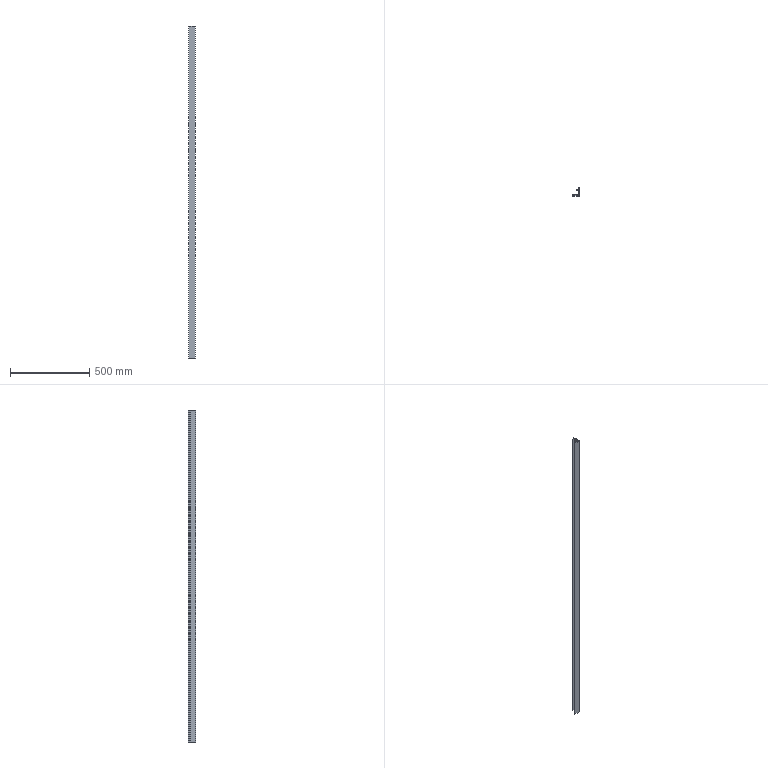Part | SolidWorks | features Extrusion 1, ICE 1 | 2 solids | 14 faces | box 43 x 50 x 2090 mm | volume 1054401 mm3 | plane 14
STEP:
#1=CARTESIAN_POINT('',(-43.,5.,-1045.));
#2=VERTEX_POINT('',#1);
#3=CARTESIAN_POINT('',(-43.,0.,-1045.));
#4=VERTEX_POINT('',#3);
#5=CARTESIAN_POINT('',(-43.,5.,-1045.));
#6=DIRECTION('',(0.,-1.,0.));
#7=VECTOR('',#6,1000.);
#8=LINE('',#5,#7);
#9=EDGE_CURVE('',#2,#4,#8,.T.);
#10=ORIENTED_EDGE('',*,*,#9,.T.);
#11=CARTESIAN_POINT('',(-43.,0.,1045.));
#12=VERTEX_POINT('',#11);
#13=CARTESIAN_POINT('',(-43.,0.,1045.));
#14=DIRECTION('',(0.,0.,-1.));
#15=VECTOR('',#14,1000.);
#16=LINE('',#13,#15);
#17=EDGE_CURVE('',#12,#4,#16,.T.);
#18=ORIENTED_EDGE('',*,*,#17,.F.);
#19=CARTESIAN_POINT('',(-43.,5.,1045.));
#20=VERTEX_POINT('',#19);
#21=CARTESIAN_POINT('',(-43.,5.,1045.));
#22=DIRECTION('',(0.,-1.,0.));
#23=VECTOR('',#22,1000.);
#24=LINE('',#21,#23);
#25=EDGE_CURVE('',#20,#12,#24,.T.);
#26=ORIENTED_EDGE('',*,*,#25,.F.);
#27=CARTESIAN_POINT('',(-43.,5.,1045.));
#28=DIRECTION('',(0.,0.,-1.));
#29=VECTOR('',#28,1000.);
#30=LINE('',#27,#29);
#31=EDGE_CURVE('',#20,#2,#30,.T.);
#32=ORIENTED_EDGE('',*,*,#31,.T.);
#33=EDGE_LOOP('',(#10,#18,#26,#32));
#34=FACE_OUTER_BOUND('',#33,.T.);
#35=CARTESIAN_POINT('',(-43.,5.,1045.));
#36=DIRECTION('',(1.,0.,0.));
#37=DIRECTION('',(0.,0.,-1.));
#38=AXIS2_PLACEMENT_3D('',#35,#36,#37);
#39=PLANE('',#38);
#40=ADVANCED_FACE('',(#34),#39,.F.);
#41=CARTESIAN_POINT('',(0.,0.,-1045.));
#42=VERTEX_POINT('',#41);
#43=CARTESIAN_POINT('',(-43.,0.,-1045.));
#44=DIRECTION('',(1.,0.,0.));
#45=VECTOR('',#44,1000.);
#46=LINE('',#43,#45);
#47=EDGE_CURVE('',#4,#42,#46,.T.);
#48=ORIENTED_EDGE('',*,*,#47,.T.);
#49=CARTESIAN_POINT('',(0.,0.,1045.));
#50=VERTEX_POINT('',#49);
#51=CARTESIAN_POINT('',(0.,0.,1045.));
#52=DIRECTION('',(0.,0.,-1.));
#53=VECTOR('',#52,1000.);
#54=LINE('',#51,#53);
#55=EDGE_CURVE('',#50,#42,#54,.T.);
#56=ORIENTED_EDGE('',*,*,#55,.F.);
#57=CARTESIAN_POINT('',(-43.,0.,1045.));
#58=DIRECTION('',(1.,0.,0.));
#59=VECTOR('',#58,1000.);
#60=LINE('',#57,#59);
#61=EDGE_CURVE('',#12,#50,#60,.T.);
#62=ORIENTED_EDGE('',*,*,#61,.F.);
#63=ORIENTED_EDGE('',*,*,#17,.T.);
#64=EDGE_LOOP('',(#48,#56,#62,#63));
#65=FACE_OUTER_BOUND('',#64,.T.);
#66=CARTESIAN_POINT('',(-43.,0.,1045.));
#67=DIRECTION('',(0.,1.,0.));
#68=DIRECTION('',(0.,0.,1.));
#69=AXIS2_PLACEMENT_3D('',#66,#67,#68);
#70=PLANE('',#69);
#71=ADVANCED_FACE('',(#65),#70,.F.);
#72=CARTESIAN_POINT('',(0.,50.,-1045.));
#73=VERTEX_POINT('',#72);
#74=CARTESIAN_POINT('',(0.,0.,-1045.));
#75=DIRECTION('',(0.,1.,0.));
#76=VECTOR('',#75,1000.);
#77=LINE('',#74,#76);
#78=EDGE_CURVE('',#42,#73,#77,.T.);
#79=ORIENTED_EDGE('',*,*,#78,.T.);
#80=CARTESIAN_POINT('',(0.,50.,1045.));
#81=VERTEX_POINT('',#80);
#82=CARTESIAN_POINT('',(0.,50.,1045.));
#83=DIRECTION('',(0.,0.,-1.));
#84=VECTOR('',#83,1000.);
#85=LINE('',#82,#84);
#86=EDGE_CURVE('',#81,#73,#85,.T.);
#87=ORIENTED_EDGE('',*,*,#86,.F.);
#88=CARTESIAN_POINT('',(0.,0.,1045.));
#89=DIRECTION('',(0.,1.,0.));
#90=VECTOR('',#89,1000.);
#91=LINE('',#88,#90);
#92=EDGE_CURVE('',#50,#81,#91,.T.);
#93=ORIENTED_EDGE('',*,*,#92,.F.);
#94=ORIENTED_EDGE('',*,*,#55,.T.);
#95=EDGE_LOOP('',(#79,#87,#93,#94));
#96=FACE_OUTER_BOUND('',#95,.T.);
#97=CARTESIAN_POINT('',(0.,0.,1045.));
#98=DIRECTION('',(-1.,0.,0.));
#99=DIRECTION('',(0.,0.,1.));
#100=AXIS2_PLACEMENT_3D('',#97,#98,#99);
#101=PLANE('',#100);
#102=ADVANCED_FACE('',(#96),#101,.F.);
#103=CARTESIAN_POINT('',(-5.,50.,-1045.));
#104=VERTEX_POINT('',#103);
#105=CARTESIAN_POINT('',(0.,50.,-1045.));
#106=DIRECTION('',(-1.,0.,0.));
#107=VECTOR('',#106,1000.);
#108=LINE('',#105,#107);
#109=EDGE_CURVE('',#73,#104,#108,.T.);
#110=ORIENTED_EDGE('',*,*,#109,.T.);
#111=CARTESIAN_POINT('',(-5.,50.,1045.));
#112=VERTEX_POINT('',#111);
#113=CARTESIAN_POINT('',(-5.,50.,1045.));
#114=DIRECTION('',(0.,0.,-1.));
#115=VECTOR('',#114,1000.);
#116=LINE('',#113,#115);
#117=EDGE_CURVE('',#112,#104,#116,.T.);
#118=ORIENTED_EDGE('',*,*,#117,.F.);
#119=CARTESIAN_POINT('',(0.,50.,1045.));
#120=DIRECTION('',(-1.,0.,0.));
#121=VECTOR('',#120,1000.);
#122=LINE('',#119,#121);
#123=EDGE_CURVE('',#81,#112,#122,.T.);
#124=ORIENTED_EDGE('',*,*,#123,.F.);
#125=ORIENTED_EDGE('',*,*,#86,.T.);
#126=EDGE_LOOP('',(#110,#118,#124,#125));
#127=FACE_OUTER_BOUND('',#126,.T.);
#128=CARTESIAN_POINT('',(0.,50.,1045.));
#129=DIRECTION('',(0.,-1.,0.));
#130=DIRECTION('',(0.,0.,-1.));
#131=AXIS2_PLACEMENT_3D('',#128,#129,#130);
#132=PLANE('',#131);
#133=ADVANCED_FACE('',(#127),#132,.F.);
#134=CARTESIAN_POINT('',(-5.,5.,-1045.));
#135=VERTEX_POINT('',#134);
#136=CARTESIAN_POINT('',(-5.,5.,-1045.));
#137=DIRECTION('',(0.,-1.,0.));
#138=VECTOR('',#137,1000.);
#139=LINE('',#136,#138);
#140=EDGE_CURVE('',#104,#135,#139,.T.);
#141=ORIENTED_EDGE('',*,*,#140,.T.);
#142=CARTESIAN_POINT('',(-5.,5.,1045.));
#143=VERTEX_POINT('',#142);
#144=CARTESIAN_POINT('',(-5.,5.,1045.));
#145=DIRECTION('',(0.,0.,-1.));
#146=VECTOR('',#145,1000.);
#147=LINE('',#144,#146);
#148=EDGE_CURVE('',#143,#135,#147,.T.);
#149=ORIENTED_EDGE('',*,*,#148,.F.);
#150=CARTESIAN_POINT('',(-5.,5.,1045.));
#151=DIRECTION('',(0.,-1.,0.));
#152=VECTOR('',#151,1000.);
#153=LINE('',#150,#152);
#154=EDGE_CURVE('',#112,#143,#153,.T.);
#155=ORIENTED_EDGE('',*,*,#154,.F.);
#156=ORIENTED_EDGE('',*,*,#117,.T.);
#157=EDGE_LOOP('',(#141,#149,#155,#156));
#158=FACE_OUTER_BOUND('',#157,.T.);
#159=CARTESIAN_POINT('',(-5.,5.,1045.));
#160=DIRECTION('',(1.,0.,0.));
#161=DIRECTION('',(0.,0.,-1.));
#162=AXIS2_PLACEMENT_3D('',#159,#160,#161);
#163=PLANE('',#162);
#164=ADVANCED_FACE('',(#158),#163,.F.);
#165=CARTESIAN_POINT('',(-43.,5.,-1045.));
#166=DIRECTION('',(-1.,0.,0.));
#167=VECTOR('',#166,1000.);
#168=LINE('',#165,#167);
#169=EDGE_CURVE('',#135,#2,#168,.T.);
#170=ORIENTED_EDGE('',*,*,#169,.T.);
#171=ORIENTED_EDGE('',*,*,#31,.F.);
#172=CARTESIAN_POINT('',(-43.,5.,1045.));
#173=DIRECTION('',(-1.,0.,0.));
#174=VECTOR('',#173,1000.);
#175=LINE('',#172,#174);
#176=EDGE_CURVE('',#143,#20,#175,.T.);
#177=ORIENTED_EDGE('',*,*,#176,.F.);
#178=ORIENTED_EDGE('',*,*,#148,.T.);
#179=EDGE_LOOP('',(#170,#171,#177,#178));
#180=FACE_OUTER_BOUND('',#179,.T.);
#181=CARTESIAN_POINT('',(-43.,5.,1045.));
#182=DIRECTION('',(0.,-1.,0.));
#183=DIRECTION('',(0.,0.,-1.));
#184=AXIS2_PLACEMENT_3D('',#181,#182,#183);
#185=PLANE('',#184);
#186=ADVANCED_FACE('',(#180),#185,.F.);
#187=ORIENTED_EDGE('',*,*,#25,.T.);
#188=ORIENTED_EDGE('',*,*,#61,.T.);
#189=ORIENTED_EDGE('',*,*,#92,.T.);
#190=ORIENTED_EDGE('',*,*,#123,.T.);
#191=ORIENTED_EDGE('',*,*,#154,.T.);
#192=ORIENTED_EDGE('',*,*,#176,.T.);
#193=EDGE_LOOP('',(#187,#188,#189,#190,#191,#192));
#194=FACE_OUTER_BOUND('',#193,.T.);
#195=CARTESIAN_POINT('',(0.,0.,1045.));
#196=DIRECTION('',(0.,0.,1.));
#197=DIRECTION('',(1.,0.,0.));
#198=AXIS2_PLACEMENT_3D('',#195,#196,#197);
#199=PLANE('',#198);
#200=ADVANCED_FACE('',(#194),#199,.T.);
#201=ORIENTED_EDGE('',*,*,#9,.F.);
#202=ORIENTED_EDGE('',*,*,#169,.F.);
#203=ORIENTED_EDGE('',*,*,#140,.F.);
#204=ORIENTED_EDGE('',*,*,#109,.F.);
#205=ORIENTED_EDGE('',*,*,#78,.F.);
#206=ORIENTED_EDGE('',*,*,#47,.F.);
#207=EDGE_LOOP('',(#201,#202,#203,#204,#205,#206));
#208=FACE_OUTER_BOUND('',#207,.T.);
#209=CARTESIAN_POINT('',(0.,0.,-1045.));
#210=DIRECTION('',(0.,0.,1.));
#211=DIRECTION('',(1.,0.,0.));
#212=AXIS2_PLACEMENT_3D('',#209,#210,#211);
#213=PLANE('',#212);
#214=ADVANCED_FACE('',(#208),#213,.F.);
#215=CLOSED_SHELL('',(#40,#71,#102,#133,#164,#186,#200,#214));
#216=MANIFOLD_SOLID_BREP('',#215);
#217=CARTESIAN_POINT('',(-5.,39.,-1045.));
#218=VERTEX_POINT('',#217);
#219=CARTESIAN_POINT('',(-5.,43.031,-1045.));
#220=VERTEX_POINT('',#219);
#221=CARTESIAN_POINT('',(-5.,39.,-1045.));
#222=DIRECTION('',(0.,1.,0.));
#223=VECTOR('',#222,1000.);
#224=LINE('',#221,#223);
#225=EDGE_CURVE('',#218,#220,#224,.T.);
#226=ORIENTED_EDGE('',*,*,#225,.T.);
#227=CARTESIAN_POINT('',(-5.,43.031,1045.));
#228=VERTEX_POINT('',#227);
#229=CARTESIAN_POINT('',(-5.,43.031,1045.));
#230=DIRECTION('',(0.,0.,-1.));
#231=VECTOR('',#230,1000.);
#232=LINE('',#229,#231);
#233=EDGE_CURVE('',#228,#220,#232,.T.);
#234=ORIENTED_EDGE('',*,*,#233,.F.);
#235=CARTESIAN_POINT('',(-5.,39.,1045.));
#236=VERTEX_POINT('',#235);
#237=CARTESIAN_POINT('',(-5.,39.,1045.));
#238=DIRECTION('',(0.,1.,0.));
#239=VECTOR('',#238,1000.);
#240=LINE('',#237,#239);
#241=EDGE_CURVE('',#236,#228,#240,.T.);
#242=ORIENTED_EDGE('',*,*,#241,.F.);
#243=CARTESIAN_POINT('',(-5.,39.,1045.));
#244=DIRECTION('',(0.,0.,-1.));
#245=VECTOR('',#244,1000.);
#246=LINE('',#243,#245);
#247=EDGE_CURVE('',#236,#218,#246,.T.);
#248=ORIENTED_EDGE('',*,*,#247,.T.);
#249=EDGE_LOOP('',(#226,#234,#242,#248));
#250=FACE_OUTER_BOUND('',#249,.T.);
#251=CARTESIAN_POINT('',(-5.,39.,1045.));
#252=DIRECTION('',(-1.,0.,0.));
#253=DIRECTION('',(0.,-1.,0.));
#254=AXIS2_PLACEMENT_3D('',#251,#252,#253);
#255=PLANE('',#254);
#256=ADVANCED_FACE('',(#250),#255,.F.);
#257=CARTESIAN_POINT('',(-21.,41.031,-1045.));
#258=VERTEX_POINT('',#257);
#259=CARTESIAN_POINT('',(-5.,43.031,-1045.));
#260=DIRECTION('',(-0.9923,-0.124,0.));
#261=VECTOR('',#260,1000.);
#262=LINE('',#259,#261);
#263=EDGE_CURVE('',#220,#258,#262,.T.);
#264=ORIENTED_EDGE('',*,*,#263,.T.);
#265=CARTESIAN_POINT('',(-21.,41.031,1045.));
#266=VERTEX_POINT('',#265);
#267=CARTESIAN_POINT('',(-21.,41.031,1045.));
#268=DIRECTION('',(0.,0.,-1.));
#269=VECTOR('',#268,1000.);
#270=LINE('',#267,#269);
#271=EDGE_CURVE('',#266,#258,#270,.T.);
#272=ORIENTED_EDGE('',*,*,#271,.F.);
#273=CARTESIAN_POINT('',(-5.,43.031,1045.));
#274=DIRECTION('',(-0.9923,-0.124,0.));
#275=VECTOR('',#274,1000.);
#276=LINE('',#273,#275);
#277=EDGE_CURVE('',#228,#266,#276,.T.);
#278=ORIENTED_EDGE('',*,*,#277,.F.);
#279=ORIENTED_EDGE('',*,*,#233,.T.);
#280=EDGE_LOOP('',(#264,#272,#278,#279));
#281=FACE_OUTER_BOUND('',#280,.T.);
#282=CARTESIAN_POINT('',(-5.,43.031,1045.));
#283=DIRECTION('',(0.124,-0.9923,0.));
#284=DIRECTION('',(0.9923,0.124,0.));
#285=AXIS2_PLACEMENT_3D('',#282,#283,#284);
#286=PLANE('',#285);
#287=ADVANCED_FACE('',(#281),#286,.F.);
#288=CARTESIAN_POINT('',(-21.,37.,-1045.));
#289=VERTEX_POINT('',#288);
#290=CARTESIAN_POINT('',(-21.,41.031,-1045.));
#291=DIRECTION('',(0.,-1.,0.));
#292=VECTOR('',#291,1000.);
#293=LINE('',#290,#292);
#294=EDGE_CURVE('',#258,#289,#293,.T.);
#295=ORIENTED_EDGE('',*,*,#294,.T.);
#296=CARTESIAN_POINT('',(-21.,37.,1045.));
#297=VERTEX_POINT('',#296);
#298=CARTESIAN_POINT('',(-21.,37.,1045.));
#299=DIRECTION('',(0.,0.,-1.));
#300=VECTOR('',#299,1000.);
#301=LINE('',#298,#300);
#302=EDGE_CURVE('',#297,#289,#301,.T.);
#303=ORIENTED_EDGE('',*,*,#302,.F.);
#304=CARTESIAN_POINT('',(-21.,41.031,1045.));
#305=DIRECTION('',(0.,-1.,0.));
#306=VECTOR('',#305,1000.);
#307=LINE('',#304,#306);
#308=EDGE_CURVE('',#266,#297,#307,.T.);
#309=ORIENTED_EDGE('',*,*,#308,.F.);
#310=ORIENTED_EDGE('',*,*,#271,.T.);
#311=EDGE_LOOP('',(#295,#303,#309,#310));
#312=FACE_OUTER_BOUND('',#311,.T.);
#313=CARTESIAN_POINT('',(-21.,41.031,1045.));
#314=DIRECTION('',(1.,0.,0.));
#315=DIRECTION('',(0.,0.,-1.));
#316=AXIS2_PLACEMENT_3D('',#313,#314,#315);
#317=PLANE('',#316);
#318=ADVANCED_FACE('',(#312),#317,.F.);
#319=CARTESIAN_POINT('',(-21.,37.,-1045.));
#320=DIRECTION('',(0.9923,0.124,0.));
#321=VECTOR('',#320,1000.);
#322=LINE('',#319,#321);
#323=EDGE_CURVE('',#289,#218,#322,.T.);
#324=ORIENTED_EDGE('',*,*,#323,.T.);
#325=ORIENTED_EDGE('',*,*,#247,.F.);
#326=CARTESIAN_POINT('',(-21.,37.,1045.));
#327=DIRECTION('',(0.9923,0.124,0.));
#328=VECTOR('',#327,1000.);
#329=LINE('',#326,#328);
#330=EDGE_CURVE('',#297,#236,#329,.T.);
#331=ORIENTED_EDGE('',*,*,#330,.F.);
#332=ORIENTED_EDGE('',*,*,#302,.T.);
#333=EDGE_LOOP('',(#324,#325,#331,#332));
#334=FACE_OUTER_BOUND('',#333,.T.);
#335=CARTESIAN_POINT('',(-21.,37.,1045.));
#336=DIRECTION('',(-0.124,0.9923,0.));
#337=DIRECTION('',(-0.9923,-0.124,0.));
#338=AXIS2_PLACEMENT_3D('',#335,#336,#337);
#339=PLANE('',#338);
#340=ADVANCED_FACE('',(#334),#339,.F.);
#341=ORIENTED_EDGE('',*,*,#241,.T.);
#342=ORIENTED_EDGE('',*,*,#277,.T.);
#343=ORIENTED_EDGE('',*,*,#308,.T.);
#344=ORIENTED_EDGE('',*,*,#330,.T.);
#345=EDGE_LOOP('',(#341,#342,#343,#344));
#346=FACE_OUTER_BOUND('',#345,.T.);
#347=CARTESIAN_POINT('',(0.,0.,1045.));
#348=DIRECTION('',(0.,0.,1.));
#349=DIRECTION('',(1.,0.,0.));
#350=AXIS2_PLACEMENT_3D('',#347,#348,#349);
#351=PLANE('',#350);
#352=ADVANCED_FACE('',(#346),#351,.T.);
#353=ORIENTED_EDGE('',*,*,#225,.F.);
#354=ORIENTED_EDGE('',*,*,#323,.F.);
#355=ORIENTED_EDGE('',*,*,#294,.F.);
#356=ORIENTED_EDGE('',*,*,#263,.F.);
#357=EDGE_LOOP('',(#353,#354,#355,#356));
#358=FACE_OUTER_BOUND('',#357,.T.);
#359=CARTESIAN_POINT('',(0.,0.,-1045.));
#360=DIRECTION('',(0.,0.,1.));
#361=DIRECTION('',(1.,0.,0.));
#362=AXIS2_PLACEMENT_3D('',#359,#360,#361);
#363=PLANE('',#362);
#364=ADVANCED_FACE('',(#358),#363,.F.);
#365=CLOSED_SHELL('',(#256,#287,#318,#340,#352,#364));
#366=MANIFOLD_SOLID_BREP('',#365);
#367=CARTESIAN_POINT('',(0.,0.,0.));
#368=DIRECTION('',(0.,0.,1.));
#369=DIRECTION('',(1.,0.,0.));
#370=AXIS2_PLACEMENT_3D('',#367,#368,#369);
#371=(LENGTH_UNIT()NAMED_UNIT(*)SI_UNIT(.MILLI.,.METRE.));
#372=UNCERTAINTY_MEASURE_WITH_UNIT(LENGTH_MEASURE(0.00001),#371,'','');
#373=(NAMED_UNIT(*)PLANE_ANGLE_UNIT()SI_UNIT($,.RADIAN.));
#374=(NAMED_UNIT(*)SI_UNIT($,.STERADIAN.)SOLID_ANGLE_UNIT());
#375=(GEOMETRIC_REPRESENTATION_CONTEXT(3)GLOBAL_UNCERTAINTY_ASSIGNED_CONTEXT((#372))GLOBAL_UNIT_ASSIGNED_CONTEXT((#371,#373,#374))REPRESENTATION_CONTEXT('',''));
#376=ADVANCED_BREP_SHAPE_REPRESENTATION('',(#216,#366,#370),#375);